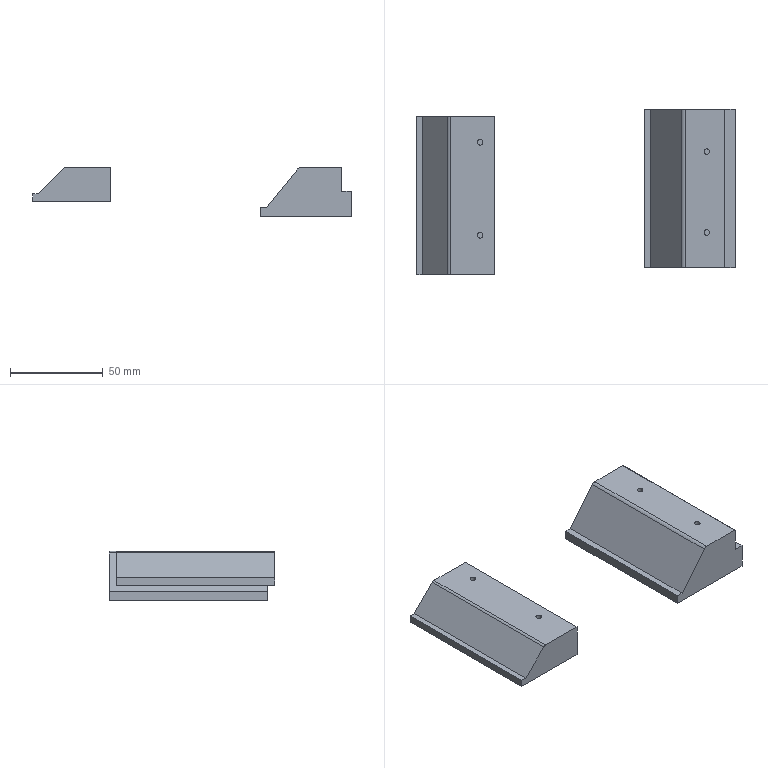NC program | NX | posted with a generic post | part box 171.319 x 88.841 x 26.598 mm
Lines 929 to 2519 of 2519:
(ZLEVEL_PROFILE , TOOL : D6R0.5)
N1838 T16 M6
N1840 G54
N1842 G17 G0 G90 X44.487 Y-6.407 S9500 M3
N1844 G43 Z30. H16
N1846 Z1.495
N1848 G94 G1 Z-0.005 F1000.
N1850 X44.029 Y-5.654
N1852 G3 X43.503 Y-5.365 R0.6
N1854 G1 X43.356 Y-5.369 F3000.
N1856 X42.665 Y-5.426
N1858 X42.5 Y-5.456
N1860 X-42.5
N1862 X-42.665 Y-5.426
N1864 X-43.356 Y-5.368
N1866 X-43.503 Y-5.365
N1868 X-43.504 Y-5.399 Z-0.01
N1870 X-42.5 Y-5.521
N1872 X42.5
N1874 X43.502 Y-5.404
N1876 X43.501 Y-5.445 Z-0.015
N1878 Y-5.478 Z-0.02
N1880 G2 X42.5 Y-5.61 R48.167
N1882 G1 X-42.5
N1884 G2 X-43.503 Y-5.463 R15.182
N1886 G1 X-43.502 Y-5.501 Z-0.025
N1888 X-43.5 Y-5.532 Z-0.03
N1890 X-42.5 Y-5.684
N1892 X42.5
N1894 X43.5 Y-5.547
N1896 Y-5.593 Z-0.037
N1898 Y-5.605 Z-0.043
N1900 G2 X42.5 Y-5.762 R67.588
N1902 G1 X-42.5
N1904 G2 X-43.5 Y-5.59 R13.651
N1906 G1 Y-5.641 Z-0.051
N1908 Y-5.658 Z-0.059
N1910 G3 X-42.5 Y-5.84 R11.561
N1912 G1 X42.5
N1914 X43.5 Y-5.675
N1916 Y-5.746 Z-0.069
N1918 Y-5.757 Z-0.078
N1920 X42.5 Y-5.92
N1922 X-42.5
N1924 X-42.665 Y-5.906
N1926 X-43.501 Y-5.74
N1928 Y-5.792 Z-0.089
N1930 Y-5.833 Z-0.1
N1932 X-42.5 Y-5.999
N1934 X42.5
N1936 X43.5 Y-5.852
N1938 Y-5.901 Z-0.113
N1940 Y-5.935 Z-0.125
N1942 X43.356 Y-5.938
N1944 X42.665 Y-6.054
N1946 X42.5 Y-6.08
N1948 X-42.5
N1950 X-43.501 Y-5.922
N1952 X-43.5 Y-5.96 Z-0.14
N1954 Y-6.013 Z-0.155
N1956 X-42.665 Y-6.145
N1958 X-42.5 Y-6.163
N1960 X42.5
N1962 X42.665 Y-6.145
N1964 X43.356 Y-6.025
N1966 X43.5 Y-6.022
N1968 Y-6.075 Z-0.171
N1970 Y-6.12 Z-0.187
N1972 X43.356 Y-6.123
N1974 X42.665 Y-6.241
N1976 X42.5 Y-6.248
N1978 X-42.5
N1980 X-42.665 Y-6.241
N1982 X-43.5 Y-6.115
N1984 Y-6.172 Z-0.206
N1986 Y-6.226 Z-0.224
N1988 X-43.356 Y-6.229
N1990 X-42.665 Y-6.323
N1992 X-42.5 Y-6.332
N1994 X42.5
N1996 X43.356 Y-6.229
N1998 X43.5 Y-6.226
N2000 Y-6.27 Z-0.244
N2002 Y-6.304 Z-0.264
N2004 X43.356 Y-6.306
N2006 X42.5 Y-6.416
N2008 X-42.5
N2010 X-43.356 Y-6.306
N2012 X-43.5 Y-6.304
N2014 Y-6.354 Z-0.286
N2016 Y-6.388 Z-0.308
N2018 X-43.356 Y-6.39
N2020 X-42.5 Y-6.5
N2022 X42.5
N2024 X43.356 Y-6.39
N2026 X43.5 Y-6.388
N2028 Y-6.435 Z-0.329
N2030 Y-6.469 Z-0.35
N2032 X43.356 Y-6.472
N2034 X42.5 Y-6.574
N2036 X-42.5
N2038 X-42.665 Y-6.569
N2040 X-43.356 Y-6.472
N2042 X-43.5 Y-6.469
N2044 Y-6.513 Z-0.371
N2046 Y-6.548 Z-0.391
N2048 G2 X-42.5 Y-6.641 R11.977
N2050 G1 X42.5
N2052 G2 X43.5 Y-6.548 R11.975
N2054 G1 Y-6.597 Z-0.416
N2056 Y-6.637 Z-0.44
N2058 X42.5 Y-6.714
N2060 X-42.5
N2062 X-43.5 Y-6.637
N2064 Y-6.677 Z-0.468
N2066 Y-6.714 Z-0.496
N2068 X-43.356 Y-6.717
N2070 X-42.665 Y-6.784
N2072 X-42.5 Y-6.792
N2074 X42.5
N2076 X42.665 Y-6.784
N2078 X43.356 Y-6.717
N2080 X43.5 Y-6.714
N2082 Y-6.755 Z-0.525
N2084 Y-6.788 Z-0.555
N2086 X43.356 Y-6.791
N2088 X42.5 Y-6.869
N2090 X-42.5
N2092 X-43.5 Y-6.79
N2094 Y-6.832 Z-0.587
N2096 Y-6.868 Z-0.618
N2098 X-42.5 Y-6.944
N2100 X42.5
N2102 X43.5 Y-6.865
N2104 Y-6.908 Z-0.651
N2106 Y-6.942 Z-0.684
N2108 X42.5 Y-7.016
N2110 X-42.5
N2112 X-43.356 Y-6.947
N2114 X-43.5 Y-6.945
N2116 Y-6.992 Z-0.717
N2118 Y-7.018 Z-0.751
N2120 X-43.356 Y-7.02
N2122 X-42.5 Y-7.084
N2124 X42.5
N2126 X43.5 Y-7.014
N2128 Y-7.062 Z-0.785
N2130 Y-7.088 Z-0.819
N2132 X43.356 Y-7.092
N2134 X42.5 Y-7.152
N2136 X-42.5
N2138 X-43.356 Y-7.094
N2140 X-43.5 Y-7.092
N2142 Y-7.139 Z-0.853
N2144 Y-7.167 Z-0.888
N2146 G2 X-42.5 Y-7.221 R12.469
N2148 G1 X42.5
N2150 X42.665 Y-7.217
N2152 X43.356 Y-7.167
N2154 X43.5 Y-7.163
N2156 Y-7.206 Z-0.923
N2158 Y-7.239 Z-0.958
N2160 X43.356 Y-7.244
N2162 X42.665 Y-7.289
N2164 X42.5 Y-7.291
N2166 X-42.5
N2168 G3 X-43.5 Y-7.243 R12.85
N2170 G1 Y-7.283 Z-0.993
N2172 Y-7.317 Z-1.028
N2174 G2 X-42.5 Y-7.362 R12.195
N2176 G1 X42.5
N2178 X42.665 Y-7.36
N2180 X43.356 Y-7.318
N2182 X43.5 Y-7.313
N2184 Y-7.351 Z-1.064
N2186 Y-7.386 Z-1.099
N2188 X43.356 Y-7.391
N2190 X42.665 Y-7.431
N2192 X42.5 Y-7.433
N2194 X-42.5
N2196 G3 X-43.5 Y-7.39 R11.828
N2198 G1 Y-7.43 Z-1.134
N2200 Y-7.463 Z-1.17
N2202 G2 X-42.5 Y-7.503 R11.483
N2204 G1 X42.5
N2206 X42.665 Y-7.502
N2208 X43.356 Y-7.464
N2210 X43.5 Y-7.46
N2212 Y-7.498 Z-1.205
N2214 Y-7.533 Z-1.241
N2216 X43.356 Y-7.537
N2218 X42.665 Y-7.572
N2220 X42.5 Y-7.574
N2222 X-42.5
N2224 G3 X-43.5 Y-7.536 R11.157
N2226 G1 Y-7.576 Z-1.276
N2228 Y-7.609 Z-1.311
N2230 G2 X-42.5 Y-7.645 R10.97
N2232 G1 X42.5
N2234 X42.665 Y-7.643
N2236 X43.356 Y-7.61
N2238 X43.5 Y-7.606
N2240 Y-7.644 Z-1.347
N2242 Y-7.679 Z-1.382
N2244 X43.356 Y-7.683
N2246 X42.665 Y-7.714
N2248 X42.5 Y-7.716
N2250 X-42.5
N2252 G3 X-43.5 Y-7.682 R11.802
N2254 G1 Y-7.722 Z-1.417
N2256 Y-7.755 Z-1.453
N2258 G2 X-42.5 Y-7.786 R12.772
N2260 G1 X42.5
N2262 X42.665 Y-7.785
N2264 X43.5 Y-7.752
N2266 Y-7.79 Z-1.488
N2268 Y-7.825 Z-1.523
N2270 X42.665 Y-7.855
N2272 X42.5 Y-7.857
N2274 X-42.5
N2276 G3 X-43.5 Y-7.828 R13.916
N2278 G1 Y-7.868 Z-1.559
N2280 Y-7.902 Z-1.594
N2282 X-43.356 Y-7.904
N2284 X-42.5 Y-7.928
N2286 X42.5
N2288 X43.5 Y-7.898
N2290 Y-7.936 Z-1.629
N2292 Y-7.971 Z-1.665
N2294 X43.356 Y-7.975
N2296 X42.5 Y-7.998
N2298 X-42.5
N2300 X-43.5 Y-7.975
N2302 Y-8.014 Z-1.7
N2304 Y-8.048 Z-1.736
N2306 X-42.5 Y-8.069
N2308 X42.5
N2310 X43.5 Y-8.044
N2312 Y-8.082 Z-1.771
N2314 Y-8.117 Z-1.806
N2316 X42.5 Y-8.14
N2318 X-42.5
N2320 X-43.5 Y-8.121
N2322 Y-8.161 Z-1.842
N2324 Y-8.194 Z-1.877
N2326 X-42.5 Y-8.211
N2328 X42.5
N2330 X43.5 Y-8.19
N2332 Y-8.228 Z-1.912
N2334 Y-8.263 Z-1.948
N2336 X42.5 Y-8.281
N2338 X-42.5
N2340 X-42.665 Y-8.276
N2342 X-43.5 Y-8.267
N2344 Y-8.307 Z-1.983
N2346 Y-8.339 Z-2.018
N2348 X-42.5 Y-8.352
N2350 X42.5
N2352 X43.356 Y-8.339
N2354 X43.5 Y-8.335
N2356 Y-8.374 Z-2.054
N2358 Y-8.407 Z-2.089
N2360 X43.356 Y-8.411
N2362 X42.5 Y-8.423
N2364 X-42.5
N2366 X-43.5 Y-8.411
N2368 Y-8.452 Z-2.124
N2370 Y-8.483 Z-2.16
N2372 X-42.5 Y-8.493
N2374 X42.5
N2376 X42.665 Y-8.492
N2378 X43.356 Y-8.483
N2380 X43.5 Y-8.479
N2382 Y-8.518 Z-2.195
N2384 Y-8.551 Z-2.23
N2386 X43.356 Y-8.555
N2388 X42.5 Y-8.564
N2390 X-42.5
N2392 X-43.5 Y-8.555
N2394 Y-8.594 Z-2.266
N2396 Y-8.627 Z-2.301
N2398 X-42.5 Y-8.635
N2400 X42.5
N2402 X43.356 Y-8.627
N2404 X43.5 Y-8.623
N2406 Y-8.66 Z-2.337
N2408 Y-8.694 Z-2.372
N2410 X43.356 Y-8.698
N2412 X42.5 Y-8.706
N2414 X-42.5
N2416 X-43.5 Y-8.698
N2418 Y-8.736 Z-2.407
N2420 Y-8.769 Z-2.443
N2422 X-42.665 Y-8.774
N2424 X-42.5 Y-8.776
N2426 X42.5
N2428 X43.356 Y-8.769
N2430 X43.5 Y-8.765
N2432 Y-8.803 Z-2.478
N2434 Y-8.837 Z-2.513
N2436 X43.356 Y-8.84
N2438 X42.5 Y-8.847
N2440 X-42.5
N2442 X-42.665 Y-8.845
N2444 X-43.5 Y-8.84
N2446 Y-8.878 Z-2.549
N2448 Y-8.911 Z-2.584
N2450 X-42.5 Y-8.918
N2452 X42.5
N2454 X43.356 Y-8.912
N2456 X43.5 Y-8.908
N2458 Y-8.945 Z-2.619
N2460 Y-8.979 Z-2.655
N2462 X43.356 Y-8.983
N2464 X42.5 Y-8.988
N2466 X-42.5
N2468 X-43.5 Y-8.983
N2470 Y-9.02 Z-2.69
N2472 Y-9.053 Z-2.725
N2474 X-42.5 Y-9.059
N2476 X42.5
N2478 X43.356 Y-9.054
N2480 X43.5 Y-9.05
N2482 Y-9.088 Z-2.761
N2484 Y-9.122 Z-2.796
N2486 X43.356 Y-9.125
N2488 X42.5 Y-9.13
N2490 X-42.5
N2492 X-42.665 Y-9.128
N2494 X-43.356 Y-9.127
N2496 X-43.5 Y-9.124
N2498 Y-9.162 Z-2.832
N2500 Y-9.195 Z-2.867
N2502 X-43.356 Y-9.198
N2504 X-42.665
N2506 X-42.5 Y-9.2
N2508 X42.5
N2510 X43.356 Y-9.197
N2512 X43.5 Y-9.193
N2514 Y-9.231 Z-2.902
N2516 Y-9.264 Z-2.938
N2518 X43.356 Y-9.268
N2520 X42.5 Y-9.271
N2522 X-42.5
N2524 X-42.665 Y-9.269
N2526 X-43.356
N2528 X-43.5 Y-9.266
N2530 Y-9.304 Z-2.973
N2532 Y-9.337 Z-3.008
N2534 X-43.356 Y-9.34
N2536 X-42.665
N2538 X-42.5 Y-9.342
N2540 X42.5
N2542 X43.356 Y-9.339
N2544 X43.5 Y-9.335
N2546 Y-9.373 Z-3.044
N2548 Y-9.406 Z-3.079
N2550 X43.356 Y-9.41
N2552 X42.5 Y-9.413
N2554 X-42.5
N2556 X-42.665 Y-9.411
N2558 X-43.356
N2560 X-43.5 Y-9.408
N2562 Y-9.446 Z-3.114
N2564 Y-9.479 Z-3.15
N2566 X-43.356 Y-9.482
N2568 X-42.5 Y-9.483
N2570 X42.5
N2572 X43.356 Y-9.481
N2574 X43.5 Y-9.478
N2576 Y-9.516 Z-3.185
N2578 Y-9.549 Z-3.22
N2580 X43.356 Y-9.552
N2582 X42.5 Y-9.554
N2584 X-42.5
N2586 X-43.356 Y-9.553
N2588 X-43.5 Y-9.55
N2590 Y-9.588 Z-3.256
N2592 Y-9.621 Z-3.291
N2594 X-43.356 Y-9.624
N2596 X-42.5 Y-9.625
N2598 X42.5
N2600 X43.356 Y-9.623
N2602 X43.5 Y-9.62
N2604 Y-9.658 Z-3.326
N2606 Y-9.691 Z-3.362
N2608 X43.356 Y-9.694
N2610 X42.5 Y-9.695
N2612 X-42.5
N2614 X-43.356 Y-9.694
N2616 X-43.5 Y-9.692
N2618 Y-9.73 Z-3.397
N2620 Y-9.762 Z-3.433
N2622 X-43.356 Y-9.765
N2624 X-42.5 Y-9.766
N2626 X42.5
N2628 X43.356 Y-9.765
N2630 X43.5 Y-9.762
N2632 Y-9.8 Z-3.468
N2634 Y-9.833 Z-3.503
N2636 X43.356 Y-9.836
N2638 X42.5 Y-9.837
N2640 X-42.5
N2642 X-43.356 Y-9.836
N2644 X-43.5 Y-9.833
N2646 Y-9.872 Z-3.539
N2648 Y-9.904 Z-3.574
N2650 X-43.356 Y-9.907
N2652 X-42.5 Y-9.908
N2654 X42.5
N2656 X43.356 Y-9.907
N2658 X43.5 Y-9.903
N2660 Y-9.942 Z-3.609
N2662 Y-9.974 Z-3.645
N2664 X43.356 Y-9.977
N2666 X42.5 Y-9.978
N2668 X-42.5
N2670 X-43.356
N2672 X-43.5 Y-9.975
N2674 Y-10.013 Z-3.68
N2676 Y-10.046 Z-3.715
N2678 X-43.356 Y-10.049
N2680 X-42.5
N2682 X42.5
N2684 X43.356 Y-10.048
N2686 X43.5 Y-10.045
N2688 Y-10.083 Z-3.751
N2690 Y-10.116 Z-3.786
N2692 X43.356 Y-10.119
N2694 X42.5 Y-10.12
N2696 X-42.5
N2698 X-43.356 Y-10.119
N2700 X-43.5 Y-10.116
N2702 Y-10.155 Z-3.821
N2704 Y-10.187 Z-3.857
N2706 X-43.356 Y-10.19
N2708 X-42.5
N2710 X42.5
N2712 X43.356
N2714 X43.5 Y-10.187
N2716 Y-10.225 Z-3.892
N2718 Y-10.258 Z-3.928
N2720 X43.356 Y-10.261
N2722 X42.5
N2724 X-42.5
N2726 X-43.356
N2728 X-43.5 Y-10.258
N2730 Y-10.296 Z-3.963
N2732 Y-10.329 Z-3.998
N2734 X-43.356 Y-10.332
N2736 X-42.5
N2738 X42.5
N2740 X43.356 Y-10.331
N2742 X43.5 Y-10.328
N2744 Y-10.367 Z-4.034
N2746 Y-10.399 Z-4.069
N2748 X43.356 Y-10.402
N2750 X42.5 Y-10.403
N2752 X-42.5
N2754 X-43.356 Y-10.402
N2756 X-43.5 Y-10.399
N2758 Y-10.438 Z-4.104
N2760 Y-10.47 Z-4.14
N2762 X-43.356 Y-10.473
N2764 X-42.5
N2766 X42.5
N2768 X43.356
N2770 X43.5 Y-10.47
N2772 Y-10.508 Z-4.175
N2774 Y-10.541 Z-4.21
N2776 X43.356 Y-10.544
N2778 X42.5
N2780 X-42.5
N2782 X-43.356
N2784 X-43.5 Y-10.541
N2786 Y-10.579 Z-4.246
N2788 Y-10.612 Z-4.281
N2790 X-43.356 Y-10.615
N2792 X-42.5
N2794 X42.5
N2796 X43.356 Y-10.614
N2798 X43.5 Y-10.611
N2800 Y-10.65 Z-4.316
N2802 Y-10.682 Z-4.352
N2804 X43.356 Y-10.685
N2806 X42.5
N2808 X-42.5
N2810 X-43.356
N2812 X-43.5 Y-10.682
N2814 Y-10.721 Z-4.387
N2816 Y-10.753 Z-4.422
N2818 X-43.356 Y-10.756
N2820 X-42.5
N2822 X42.5
N2824 X43.356
N2826 X43.5 Y-10.753
N2828 Y-10.791 Z-4.458
N2830 Y-10.824 Z-4.493
N2832 X43.356 Y-10.827
N2834 X42.5
N2836 X-42.5
N2838 X-43.356
N2840 X-43.5 Y-10.824
N2842 Y-10.862 Z-4.529
N2844 Y-10.894 Z-4.564
N2846 X-43.356 Y-10.897
N2848 X-42.5 Y-10.898
N2850 X42.5
N2852 X43.356 Y-10.897
N2854 X43.5 Y-10.894
N2856 Y-10.933 Z-4.599
N2858 Y-10.965 Z-4.635
N2860 X43.356 Y-10.968
N2862 X42.5
N2864 X-42.5
N2866 X-43.356
N2868 X-43.5 Y-10.965
N2870 Y-11.004 Z-4.67
N2872 Y-11.036 Z-4.705
N2874 X-43.356 Y-11.039
N2876 X-42.5
N2878 X42.5
N2880 X43.356
N2882 X43.5 Y-11.036
N2884 Y-11.074 Z-4.741
N2886 Y-11.107 Z-4.776
N2888 X43.356 Y-11.11
N2890 X42.5
N2892 X-42.5
N2894 X-43.356
N2896 X-43.5 Y-11.107
N2898 Y-11.145 Z-4.811
N2900 Y-11.177 Z-4.847
N2902 X-43.356 Y-11.18
N2904 X-42.5
N2906 X42.5
N2908 X43.356
N2910 X43.5 Y-11.177
N2912 Y-11.216 Z-4.882
N2914 Y-11.248 Z-4.917
N2916 X43.356 Y-11.251
N2918 X42.5
N2920 X-42.5
N2922 X-43.356
N2924 X-43.5 Y-11.248
N2926 Y-11.286 Z-4.953
N2928 Y-11.319 Z-4.988
N2930 X-43.356 Y-11.322
N2932 X-42.5
N2934 X42.5
N2936 X43.356
N2938 X43.5 Y-11.319
N2940 Y-11.357 Z-5.024
N2942 Y-11.39 Z-5.059
N2944 X43.356 Y-11.392
N2946 X42.5 Y-11.393
N2948 X-42.5
N2950 X-43.356
N2952 X-43.5 Y-11.39
N2954 Y-11.428 Z-5.094
N2956 Y-11.46 Z-5.13
N2958 X-43.356 Y-11.463
N2960 X-42.5
N2962 X42.5
N2964 X43.356
N2966 X43.5 Y-11.46
N2968 Y-11.499 Z-5.165
N2970 Y-11.531 Z-5.2
N2972 X43.356 Y-11.534
N2974 X42.5
N2976 X-42.5
N2978 X-43.356
N2980 X-43.5 Y-11.531
N2982 Y-11.569 Z-5.236
N2984 Y-11.602 Z-5.271
N2986 X-43.356 Y-11.605
N2988 X-42.5
N2990 X42.5
N2992 X43.356
N2994 X43.5 Y-11.602
N2996 Y-11.64 Z-5.306
N2998 Y-11.672 Z-5.342
N3000 X43.356 Y-11.675
N3002 X42.5
N3004 X-42.5
N3006 X-43.356
N3008 X-43.5 Y-11.672
N3010 Y-11.711 Z-5.377
N3012 Y-11.744 Z-5.412
N3014 X-43.356 Y-11.746
N3016 X-42.5
N3018 X42.5
N3020 X43.356
N3022 X43.5 Y-11.744
N3024 Y-11.781 Z-5.448
N3026 Y-11.814 Z-5.483
N3028 X43.356 Y-11.817
N3030 X42.5
N3032 X-42.5
N3034 X-43.356
N3036 X-43.5 Y-11.814
N3038 Y-11.852 Z-5.518
N3040 Y-11.885 Z-5.554
N3042 X-43.356 Y-11.888
N3044 X-42.5
N3046 X42.5
N3048 X43.356
N3050 X43.5 Y-11.885
N3052 Y-11.923 Z-5.589
N3054 Y-11.955 Z-5.625
N3056 X43.356 Y-11.958
N3058 X42.5
N3060 X-42.5
N3062 X-43.356
N3064 X-43.5 Y-11.955
N3066 Y-11.994 Z-5.66
N3068 Y-12.026 Z-5.695
N3070 X-43.356 Y-12.029
N3072 X-42.5
N3074 X42.5
N3076 X43.356
N3078 X43.5 Y-12.026
N3080 Y-12.064 Z-5.731
N3082 Y-12.097 Z-5.766
N3084 X43.356 Y-12.1
N3086 X42.5
N3088 X-42.5
N3090 X-43.356
N3092 X-43.5 Y-12.097
N3094 Y-12.135 Z-5.801
N3096 Y-12.167 Z-5.837
N3098 X-43.356 Y-12.17
N3100 X-42.5
N3102 X42.5
N3104 X43.356
N3106 X43.5 Y-12.167
N3108 Y-12.206 Z-5.872
N3110 Y-12.238 Z-5.907
N3112 X43.356 Y-12.241
N3114 X42.5
N3116 X-42.5
N3118 X-43.356
N3120 X-43.5 Y-12.238
N3122 Y-12.276 Z-5.943
N3124 Y-12.309 Z-5.978
N3126 X-43.356 Y-12.312
N3128 X-42.5
N3130 X42.5
N3132 X43.356
N3134 X43.5 Y-12.309
N3136 Y-12.347 Z-6.013
N3138 Y-12.38 Z-6.049
N3140 X43.356 Y-12.383
N3142 X42.5
N3144 X-42.5
N3146 X-43.356
N3148 X-43.5 Y-12.38
N3150 Y-12.418 Z-6.084
N3152 Y-12.45 Z-6.12
N3154 X-43.356 Y-12.453
N3156 X-42.5
N3158 X42.5
N3160 X43.356
N3162 X43.5 Y-12.45
N3164 Y-12.489 Z-6.155
N3166 Y-12.521 Z-6.19
N3168 X43.356 Y-12.524
N3170 X42.5
N3172 X-42.5
N3174 X-43.356
N3176 X-43.5 Y-12.521
N3178 Y-12.559 Z-6.226
N3180 Y-12.592 Z-6.261
N3182 X-43.356 Y-12.595
N3184 X-42.5
N3186 X42.5
N3188 X43.356
N3190 X43.5 Y-12.592
N3192 Y-12.63 Z-6.296
N3194 Y-12.662 Z-6.332
N3196 X43.356 Y-12.665
N3198 X42.5
N3200 X-42.5
N3202 X-43.356
N3204 X-43.5 Y-12.662
N3206 Y-12.701 Z-6.367
N3208 Y-12.733 Z-6.402
N3210 X-43.356 Y-12.736
N3212 X-42.5
N3214 X42.5
N3216 X43.356
N3218 X43.5 Y-12.733
N3220 Y-12.771 Z-6.438
N3222 Y-12.804 Z-6.473
N3224 X43.356 Y-12.807
N3226 X42.5
N3228 X-42.5
N3230 X-43.356
N3232 X-43.5 Y-12.804
N3234 Y-12.842 Z-6.508
N3236 Y-12.875 Z-6.544
N3238 X-43.356 Y-12.877
N3240 X-42.5
N3242 X42.5
N3244 X43.356
N3246 X43.5 Y-12.875
N3248 Y-12.913 Z-6.579
N3250 Y-12.945 Z-6.614
N3252 X43.356 Y-12.948
N3254 X42.5
N3256 X-42.5
N3258 X-43.356
N3260 X-43.5 Y-12.945
N3262 Y-12.984 Z-6.65
N3264 Y-13.016 Z-6.685
N3266 X-43.356 Y-13.019
N3268 X-42.5
N3270 X42.5
N3272 X43.356
N3274 X43.5 Y-13.016
N3276 Y-13.054 Z-6.721
N3278 Y-13.087 Z-6.756
N3280 X43.356 Y-13.09
N3282 X42.5
N3284 X-42.5
N3286 X-43.356
N3288 X-43.5 Y-13.087
N3290 Y-13.125 Z-6.791
N3292 Y-13.157 Z-6.827
N3294 X-43.356 Y-13.16
N3296 X-42.5
N3298 X42.5
N3300 X43.356
N3302 X43.5 Y-13.157
N3304 Y-13.196 Z-6.862
N3306 Y-13.228 Z-6.897
N3308 X43.356 Y-13.231
N3310 X42.5
N3312 X-42.5
N3314 X-43.356
N3316 X-43.5 Y-13.228
N3318 Y-13.266 Z-6.933
N3320 Y-13.299 Z-6.968
N3322 X-43.356 Y-13.302
N3324 X-42.5
N3326 X42.5
N3328 X43.356
N3330 X43.5 Y-13.299
N3332 Y-13.337 Z-7.003
N3334 Y-13.37 Z-7.039
N3336 X43.356 Y-13.372
N3338 X42.5
N3340 X-42.5
N3342 X-43.356
N3344 X-43.5 Y-13.37
N3346 Y-13.408 Z-7.074
N3348 Y-13.44 Z-7.109
N3350 X-43.356 Y-13.443
N3352 X-42.5
N3354 X42.5
N3356 X43.356
N3358 X43.5 Y-13.44
N3360 Y-13.479 Z-7.145
N3362 Y-13.511 Z-7.18
N3364 X43.356 Y-13.514
N3366 X42.5
N3368 X-42.5
N3370 X-43.356
N3372 X-43.5 Y-13.511
N3374 Y-13.549 Z-7.216
N3376 Y-13.582 Z-7.251
N3378 X-43.356 Y-13.585
N3380 X-42.5
N3382 X42.5
N3384 X43.356
N3386 X43.5 Y-13.582
N3388 Y-13.62 Z-7.286
N3390 Y-13.652 Z-7.322
N3392 X43.356 Y-13.655
N3394 X42.5
N3396 X-42.5
N3398 X-43.356
N3400 X-43.5 Y-13.652
N3402 Y-13.691 Z-7.357
N3404 Y-13.723 Z-7.392
N3406 X-43.356 Y-13.726
N3408 X-42.5
N3410 X42.5
N3412 X43.356
N3414 X43.5 Y-13.723
N3416 Y-13.761 Z-7.428
N3418 Y-13.794 Z-7.463
N3420 X43.356 Y-13.797
N3422 X42.5
N3424 X-42.5
N3426 X-43.356
N3428 X-43.5 Y-13.794
N3430 Y-13.832 Z-7.498
N3432 Y-13.864 Z-7.534
N3434 X-43.356 Y-13.867
N3436 X-42.5
N3438 X42.5
N3440 X43.356
N3442 X43.5 Y-13.864
N3444 Y-13.903 Z-7.569
N3446 Y-13.935 Z-7.604
N3448 X43.356 Y-13.938
N3450 X42.5
N3452 X-42.5
N3454 X-43.356
N3456 X-43.5 Y-13.935
N3458 Y-13.974 Z-7.64
N3460 Y-14.006 Z-7.675
N3462 X-43.356 Y-14.009
N3464 X-42.5
N3466 X42.5
N3468 X43.356
N3470 X43.5 Y-14.006
N3472 Y-14.044 Z-7.711
N3474 Y-14.077 Z-7.746
N3476 X43.356 Y-14.08
N3478 X42.5
N3480 X-42.5
N3482 X-43.356
N3484 X-43.5 Y-14.077
N3486 Y-14.115 Z-7.781
N3488 X-43.499 Y-14.147 Z-7.817
N3490 X-43.356 Y-14.15
N3492 X-42.5
N3494 X42.5
N3496 X43.356
N3498 X43.5 Y-14.147
N3500 Y-14.186 Z-7.852
N3502 Y-14.218 Z-7.887
N3504 X43.356 Y-14.221
N3506 X42.5
N3508 X-42.5
N3510 X-43.356
N3512 X-43.499 Y-14.218
N3514 Y-14.256 Z-7.923
N3516 Y-14.289 Z-7.958
N3518 X-43.356 Y-14.292
N3520 X-42.5
N3522 X42.5
N3524 X43.356
N3526 X43.5 Y-14.289
N3528 Y-14.327 Z-7.993
N3530 Y-14.359 Z-8.029
N3532 X43.356 Y-14.362
N3534 X42.5
N3536 X-42.5
N3538 X-43.356
N3540 X-43.499 Y-14.359
N3542 Y-14.398 Z-8.064
N3544 Y-14.43 Z-8.099
N3546 X-43.356 Y-14.433
N3548 X-42.5
N3550 X42.5
N3552 X43.356
N3554 X43.5 Y-14.43
N3556 Y-14.468 Z-8.135
N3558 X43.499 Y-14.501 Z-8.17
N3560 X43.356 Y-14.504
N3562 X42.5
N3564 X-42.5
N3566 X-43.356
N3568 X-43.499 Y-14.501
N3570 Y-14.539 Z-8.205
N3572 Y-14.572 Z-8.241
N3574 X-43.356 Y-14.575
N3576 X-42.5
N3578 X42.5
N3580 X43.356
N3582 X43.499 Y-14.572
N3584 Y-14.61 Z-8.276
N3586 Y-14.642 Z-8.312
N3588 X43.356 Y-14.645
N3590 X42.5
N3592 X-42.5
N3594 X-43.356
N3596 X-43.499 Y-14.642
N3598 Y-14.681 Z-8.347
N3600 Y-14.713 Z-8.382
N3602 X-43.356 Y-14.716
N3604 X-42.5
N3606 X42.5
N3608 X43.356
N3610 X43.499 Y-14.713
N3612 Y-14.751 Z-8.418
N3614 Y-14.784 Z-8.453
N3616 X43.356 Y-14.787
N3618 X-43.356
N3620 X-43.499 Y-14.784
N3622 Y-14.822 Z-8.488
N3624 Y-14.854 Z-8.524
N3626 X-43.356 Y-14.857
N3628 X43.356
N3630 X43.499 Y-14.854
N3632 Y-14.893 Z-8.559
N3634 Y-14.925 Z-8.594
N3636 X43.356 Y-14.928
N3638 X-43.356
N3640 X-43.499 Y-14.925
N3642 Y-14.963 Z-8.63
N3644 Y-14.996 Z-8.665
N3646 X-43.356 Y-14.999
N3648 X43.356
N3650 X43.499 Y-14.996
N3652 Y-15.034 Z-8.7
N3654 Y-15.067 Z-8.736
N3656 X43.356 Y-15.07
N3658 X-43.356
N3660 X-43.499 Y-15.067
N3662 Y-15.105 Z-8.771
N3664 Y-15.137 Z-8.807
N3666 X-43.356 Y-15.14
N3668 X43.356
N3670 X43.499 Y-15.137
N3672 Y-15.176 Z-8.842
N3674 Y-15.208 Z-8.877
N3676 X43.356 Y-15.211
N3678 X-43.356
N3680 X-43.499 Y-15.208
N3682 Y-15.246 Z-8.913
N3684 Y-15.279 Z-8.948
N3686 X-43.356 Y-15.282
N3688 X42.5
N3690 X43.356
N3692 X43.499 Y-15.279
N3694 Y-15.317 Z-8.983
N3696 Y-15.349 Z-9.019
N3698 X43.356 Y-15.352
N3700 X42.5
N3702 X-43.356
N3704 X-43.499 Y-15.349
N3706 Y-15.388 Z-9.054
N3708 Y-15.42 Z-9.089
N3710 X-43.356 Y-15.423
N3712 X42.5
N3714 X43.356
N3716 X43.499 Y-15.42
N3718 Y-15.458 Z-9.125
N3720 Y-15.491 Z-9.16
N3722 X43.356 Y-15.494
N3724 X42.5
N3726 X-43.356
N3728 X-43.499 Y-15.491
N3730 Y-15.529 Z-9.195
N3732 Y-15.562 Z-9.231
N3734 X-43.356 Y-15.565
N3736 X42.5
N3738 X43.356
N3740 X43.499 Y-15.562
N3742 Y-15.6 Z-9.266
N3744 Y-15.632 Z-9.301
N3746 X43.356 Y-15.635
N3748 X42.5
N3750 X-43.356
N3752 X-43.499 Y-15.632
N3754 Y-15.671 Z-9.337
N3756 Y-15.703 Z-9.372
N3758 X-43.356 Y-15.706
N3760 X42.5
N3762 X43.356
N3764 X43.499 Y-15.703
N3766 Y-15.741 Z-9.408
N3768 Y-15.774 Z-9.443
N3770 X43.356 Y-15.777
N3772 X42.5
N3774 X-43.356
N3776 X-43.499 Y-15.774
N3778 Y-15.812 Z-9.478
N3780 Y-15.844 Z-9.514
N3782 X-43.356 Y-15.847
N3784 X42.5
N3786 X43.356
N3788 X43.499 Y-15.844
N3790 X43.498 Y-15.883 Z-9.549
N3792 Y-15.915 Z-9.584
N3794 X43.356 Y-15.918
N3796 X42.5
N3798 X-43.356
N3800 X-43.498 Y-15.915
N3802 Y-15.953 Z-9.62
N3804 Y-15.986 Z-9.655
N3806 X-43.356 Y-15.989
N3808 X42.5
N3810 X43.356
N3812 X43.498 Y-15.986
N3814 Y-16.024 Z-9.69
N3816 Y-16.057 Z-9.726
N3818 X43.356 Y-16.06
N3820 X42.5
N3822 X-43.356
N3824 X-43.498 Y-16.057
N3826 Y-16.095 Z-9.761
N3828 Y-16.127 Z-9.796
N3830 X-43.356 Y-16.13
N3832 X42.5
N3834 X43.356
N3836 X43.498 Y-16.127
N3838 Y-16.166 Z-9.832
N3840 Y-16.198 Z-9.867
N3842 X43.356 Y-16.201
N3844 X42.5
N3846 X-43.356
N3848 X-43.498 Y-16.198
N3850 Y-16.236 Z-9.903
N3852 Y-16.269 Z-9.938
N3854 X-43.356 Y-16.272
N3856 X42.5
N3858 X43.356
N3860 X43.498 Y-16.269
N3862 Y-16.307 Z-9.973
N3864 Y-16.339 Z-10.009
N3866 X43.356 Y-16.342
N3868 X42.5
N3870 X-43.356
N3872 X-43.498 Y-16.339
N3874 Y-16.378 Z-10.044
N3876 Y-16.41 Z-10.079
N3878 X-43.356 Y-16.413
N3880 X42.5
N3882 X43.356
N3884 X43.498 Y-16.41
N3886 Y-16.448 Z-10.115
N3888 Y-16.481 Z-10.15
N3890 X43.356 Y-16.484
N3892 X42.5
N3894 X-43.356
N3896 X-43.498 Y-16.481
N3898 Y-16.519 Z-10.185
N3900 Y-16.552 Z-10.221
N3902 X-43.356 Y-16.554
N3904 X42.5
N3906 X43.356
N3908 X43.498 Y-16.552
N3910 Y-16.59 Z-10.256
N3912 X43.497 Y-16.622 Z-10.291
N3914 X43.356 Y-16.625
N3916 X42.5
N3918 X-43.356
N3920 X-43.498 Y-16.622
N3922 X-43.497 Y-16.661 Z-10.327
N3924 Y-16.693 Z-10.362
N3926 X-43.356 Y-16.696
N3928 X42.5
N3930 X43.356
N3932 X43.497 Y-16.693
N3934 Y-16.731 Z-10.397
N3936 Y-16.764 Z-10.433
N3938 X43.356 Y-16.767
N3940 X42.5
N3942 X-43.356
N3944 X-43.497 Y-16.764
N3946 Y-16.802 Z-10.468
N3948 Y-16.834 Z-10.504
N3950 X-43.356 Y-16.837
N3952 X42.5
N3954 X43.356
N3956 X43.497 Y-16.834
N3958 Y-16.873 Z-10.539
N3960 Y-16.905 Z-10.574
N3962 X43.356 Y-16.908
N3964 X42.5
N3966 X-43.356
N3968 X-43.497 Y-16.905
N3970 Y-16.943 Z-10.61
N3972 Y-16.976 Z-10.645
N3974 X-43.356 Y-16.979
N3976 X42.5
N3978 X43.356
N3980 X43.497 Y-16.976
N3982 Y-17.014 Z-10.68
N3984 X43.496 Y-17.046 Z-10.716
N3986 X43.356 Y-17.049
N3988 X42.5
N3990 X-43.356
N3992 X-43.496 Y-17.046
N3994 Y-17.085 Z-10.751
N3996 Y-17.117 Z-10.786
N3998 X-43.356 Y-17.12
N4000 X42.5
N4002 X43.356
N4004 X43.496 Y-17.117
N4006 Y-17.156 Z-10.822
N4008 Y-17.188 Z-10.857
N4010 X43.356 Y-17.191
N4012 X42.5
N4014 X-43.356
N4016 X-43.496 Y-17.188
N4018 Y-17.226 Z-10.892
N4020 Y-17.259 Z-10.928
N4022 X-43.356 Y-17.262
N4024 X42.5
N4026 X43.356
N4028 X43.496 Y-17.259
N4030 Y-17.297 Z-10.963
N4032 Y-17.329 Z-10.999
N4034 X43.356 Y-17.332
N4036 X42.5
N4038 X-43.356
N4040 X-43.496 Y-17.329
N4042 X-43.495 Y-17.368 Z-11.034
N4044 Y-17.4 Z-11.069
N4046 X-43.356 Y-17.403
N4048 X42.5
N4050 X43.356
N4052 X43.495 Y-17.4
N4054 Y-17.438 Z-11.105
N4056 Y-17.471 Z-11.14
N4058 X43.356 Y-17.474
N4060 X42.5
N4062 X-43.356
N4064 X-43.495 Y-17.471
N4066 Y-17.509 Z-11.175
N4068 Y-17.541 Z-11.211
N4070 X-43.356 Y-17.544
N4072 X42.5
N4074 X43.356
N4076 X43.495 Y-17.541
N4078 Y-17.58 Z-11.246
N4080 Y-17.613 Z-11.281
N4082 X43.356 Y-17.615
N4084 X42.5
N4086 X-43.356
N4088 X-43.495 Y-17.613
N4090 Y-17.651 Z-11.317
N4092 Y-17.683 Z-11.352
N4094 X-43.356 Y-17.686
N4096 X42.5
N4098 X43.356
N4100 X43.495 Y-17.683
N4102 Y-17.721 Z-11.387
N4104 X43.494 Y-17.754 Z-11.423
N4106 X43.356 Y-17.757
N4108 X42.5
N4110 X-43.356
N4112 X-43.494 Y-17.754
N4114 Y-17.792 Z-11.458
N4116 Y-17.824 Z-11.493
N4118 X-43.356 Y-17.827
N4120 X42.5
N4122 X43.356
N4124 X43.494 Y-17.824
N4126 Y-17.863 Z-11.529
N4128 Y-17.895 Z-11.564
N4130 X43.356 Y-17.898
N4132 X42.5
N4134 X-43.356
N4136 X-43.494 Y-17.895
N4138 Y-17.933 Z-11.6
N4140 Y-17.966 Z-11.635
N4142 X-43.356 Y-17.969
N4144 X42.5
N4146 X43.356
N4148 X43.494 Y-17.966
N4150 Y-18.004 Z-11.67
N4152 X43.493 Y-18.036 Z-11.706
N4154 X43.356 Y-18.039
N4156 X42.5
N4158 X-43.356
N4160 X-43.493 Y-18.036
N4162 Y-18.075 Z-11.741
N4164 Y-18.107 Z-11.776
N4166 X-43.356 Y-18.11
N4168 X42.5
N4170 X43.356
N4172 X43.493 Y-18.107
N4174 Y-18.145 Z-11.812
N4176 Y-18.178 Z-11.847
N4178 X43.356 Y-18.181
N4180 X42.5
N4182 X-43.356
N4184 X-43.493 Y-18.178
N4186 X-43.492 Y-18.216 Z-11.882
N4188 Y-18.249 Z-11.918
N4190 X-43.356 Y-18.252
N4192 X42.5
N4194 X43.356
N4196 X43.492 Y-18.249
N4198 Y-18.287 Z-11.953
N4200 Y-18.319 Z-11.988
N4202 X43.356 Y-18.322
N4204 X42.5
N4206 X-43.356
N4208 X-43.492 Y-18.319
N4210 Y-18.358 Z-12.024
N4212 Y-18.39 Z-12.059
N4214 X-43.356 Y-18.393
N4216 X42.5
N4218 X43.356
N4220 X43.492 Y-18.39
N4222 X43.491 Y-18.428 Z-12.095
N4224 Y-18.461 Z-12.13
N4226 X43.356 Y-18.464
N4228 X42.5
N4230 X-43.356
N4232 X-43.491 Y-18.461
N4234 Y-18.499 Z-12.165
N4236 Y-18.531 Z-12.201
N4238 X-43.356 Y-18.534
N4240 X42.5
N4242 X43.356
N4244 X43.491 Y-18.531
N4246 Y-18.57 Z-12.236
N4248 X43.49 Y-18.602 Z-12.271
N4250 X43.356 Y-18.605
N4252 X42.5
N4254 X-43.356
N4256 X-43.49 Y-18.602
N4258 Y-18.64 Z-12.307
N4260 Y-18.673 Z-12.342
N4262 X-43.356 Y-18.676
N4264 X42.5
N4266 X43.356
N4268 X43.49 Y-18.673
N4270 Y-18.711 Z-12.377
N4272 Y-18.743 Z-12.413
N4274 X43.356 Y-18.747
N4276 X42.5
N4278 X-43.356
N4280 X-43.489 Y-18.744
N4282 Y-18.782 Z-12.448
N4284 Y-18.814 Z-12.483
N4286 X-43.356 Y-18.817
N4288 X42.5
N4290 X43.356
N4292 X43.489 Y-18.814
N4294 Y-18.853 Z-12.519
N4296 Y-18.885 Z-12.554
N4298 X43.356 Y-18.888
N4300 X42.5
N4302 X-43.356
N4304 X-43.489 Y-18.885
N4306 X-43.488 Y-18.923 Z-12.589
N4308 Y-18.956 Z-12.625
N4310 X-43.356 Y-18.959
N4312 X42.5
N4314 X43.356
N4316 X43.488 Y-18.956
N4318 Y-18.994 Z-12.66
N4320 Y-19.026 Z-12.696
N4322 X43.356 Y-19.029
N4324 X42.5
N4326 X-43.356
N4328 X-43.488 Y-19.026
N4330 Y-19.065 Z-12.731
N4332 X-43.487 Y-19.097 Z-12.766
N4334 X-43.356 Y-19.1
N4336 X42.5
N4338 X43.356
N4340 X43.487 Y-19.097
N4342 Y-19.135 Z-12.802
N4344 Y-19.168 Z-12.837
N4346 X43.356 Y-19.171
N4348 X42.5
N4350 X-43.356
N4352 X-43.487 Y-19.168
N4354 Y-19.206 Z-12.872
N4356 Y-19.238 Z-12.908
N4358 X-43.356 Y-19.242
N4360 X42.5
N4362 X43.356
N4364 X43.487 Y-19.238
N4366 X43.486 Y-19.277 Z-12.943
N4368 Y-19.309 Z-12.978
N4370 X43.356 Y-19.312
N4372 X42.5
N4374 X-43.356
N4376 X-43.486 Y-19.309
N4378 Y-19.348 Z-13.014
N4380 Y-19.38 Z-13.049
N4382 X-43.356 Y-19.383
N4384 X42.5
N4386 X43.356
N4388 X43.486 Y-19.38
N4390 X43.485 Y-19.418 Z-13.084
N4392 Y-19.451 Z-13.12
N4394 X43.356 Y-19.454
N4396 X42.5
N4398 X-43.356
N4400 X-43.485 Y-19.451
N4402 Y-19.489 Z-13.155
N4404 Y-19.521 Z-13.191
N4406 X-43.356 Y-19.524
N4408 X42.5
N4410 X43.356
N4412 X43.485 Y-19.521
N4414 Y-19.56 Z-13.226
N4416 X43.484 Y-19.592 Z-13.261
N4418 X43.356 Y-19.595
N4420 X42.5
N4422 X-43.356
N4424 X-43.484 Y-19.592
N4426 Y-19.63 Z-13.297
N4428 Y-19.663 Z-13.332
N4430 X-43.356 Y-19.666
N4432 X42.5
N4434 X43.356
N4436 X43.484 Y-19.663
N4438 Y-19.701 Z-13.367
N4440 X43.483 Y-19.733 Z-13.403
N4442 X43.356 Y-19.737
N4444 X42.5
N4446 X-43.356
N4448 X-43.483 Y-19.733
N4450 Y-19.772 Z-13.438
N4452 Y-19.804 Z-13.473
N4454 X-43.356 Y-19.807
N4456 X42.5
N4458 X43.356
N4460 X43.483 Y-19.804
N4462 X43.482 Y-19.843 Z-13.509
N4464 Y-19.875 Z-13.544
N4466 X43.356 Y-19.878
N4468 X42.5
N4470 X-43.356
N4472 X-43.482 Y-19.875
N4474 Y-19.913 Z-13.579
N4476 Y-19.946 Z-13.615
N4478 X-43.356 Y-19.949
N4480 X42.5
N4482 X43.356
N4484 X43.482 Y-19.946
N4486 X43.481 Y-19.984 Z-13.65
N4488 Y-20.016 Z-13.685
N4490 X43.356 Y-20.019
N4492 X42.5
N4494 X-43.356
N4496 X-43.481 Y-20.016
N4498 Y-20.055 Z-13.721
N4500 X-43.48 Y-20.087 Z-13.756
N4502 X-43.356 Y-20.09
N4504 X42.5
N4506 X43.356
N4508 X43.481 Y-20.087
N4510 X43.48 Y-20.125 Z-13.792
N4512 Y-20.158 Z-13.827
N4514 X43.356 Y-20.161
N4516 X42.5
N4518 X-43.356
N4520 X-43.48 Y-20.158
N4522 Y-20.196 Z-13.862
N4524 X-43.479 Y-20.228 Z-13.898
N4526 X-43.356 Y-20.231
N4528 X42.5
N4530 X43.356
N4532 X43.479 Y-20.228
N4534 Y-20.267 Z-13.933
N4536 Y-20.299 Z-13.968
N4538 X43.356 Y-20.302
N4540 X42.5
N4542 X-43.356
N4544 X-43.479 Y-20.299
N4546 X-43.478 Y-20.338 Z-14.004
N4548 X-43.477 Y-20.371 Z-14.039
N4550 X-43.356 Y-20.373
N4552 X-42.5
N4554 X42.5
N4556 X43.356
N4558 X43.477 Y-20.371
N4560 X43.447 Y-20.436 Z-14.105
N4562 X43.356 Y-20.439
N4564 X42.5
N4566 X-42.5
N4568 X-43.356
N4570 X-43.447 Y-20.436
N4572 X-43.417 Y-20.503 Z-14.171
N4574 X-43.356 Y-20.505
N4576 X-42.5 Y-20.504
N4578 X42.5
N4580 X43.356 Y-20.505
N4582 X43.417 Y-20.503
N4584 X43.386 Y-20.57 Z-14.236
N4586 X42.5
N4588 X-42.5
N4590 X-43.386
N4592 X-43.357 Y-20.634 Z-14.302
N4594 X-42.5 Y-20.633
N4596 X42.5
N4598 X43.357 Y-20.634
N4600 G2 X43.877 Y-20.934 R0.6
N4602 G1 X44.341 Y-21.739
N4604 Z-12.802
N4606 G0 Z30.
N4608 M5
(HOLE_MILLING , TOOL : D2)
N4610 T17 M6
N4612 G54
N4614 G17 G0 G90 X-28.65 Y13.086 S9500 M3
N4616 G43 Z30. H17
N4618 Z0.5
N4620 G94 G3 X-28.45 Y13.286 R0.2 F1000.
N4622 X-28.65 Y13.486 R0.2
N4624 X-28.65 Y13.486 Z0.35 I0. J-0.4
N4626 X-28.65 Y13.486 Z0.2 I0. J-0.4
N4628 X-28.65 Y13.486 Z0.05 I0. J-0.4
N4630 X-28.65 Y13.486 Z-0.1 I0. J-0.4
N4632 X-28.65 Y13.486 Z-0.25 I0. J-0.4
N4634 X-28.65 Y13.486 Z-0.4 I0. J-0.4
N4636 X-28.65 Y13.486 Z-0.55 I0. J-0.4
N4638 X-28.65 Y13.486 Z-0.7 I0. J-0.4
N4640 X-28.65 Y13.486 Z-0.85 I0. J-0.4
N4642 X-28.65 Y13.486 Z-1. I0. J-0.4
N4644 X-28.65 Y13.486 Z-1.15 I0. J-0.4
N4646 X-28.65 Y13.486 Z-1.3 I0. J-0.4
N4648 X-28.65 Y13.486 Z-1.45 I0. J-0.4
N4650 X-28.65 Y13.486 Z-1.6 I0. J-0.4
N4652 X-28.65 Y13.486 Z-1.75 I0. J-0.4
N4654 X-28.65 Y13.486 Z-1.9 I0. J-0.4
N4656 X-28.65 Y13.486 Z-2.05 I0. J-0.4
N4658 X-28.65 Y13.486 Z-2.2 I0. J-0.4
N4660 X-28.65 Y13.486 Z-2.35 I0. J-0.4
N4662 X-28.65 Y13.486 Z-2.5 I0. J-0.4
N4664 X-28.65 Y13.486 Z-2.65 I0. J-0.4
N4666 X-28.65 Y13.486 Z-2.8 I0. J-0.4
N4668 X-28.65 Y13.486 Z-2.95 I0. J-0.4
N4670 X-28.65 Y13.486 Z-3.1 I0. J-0.4
N4672 X-28.65 Y13.486 Z-3.25 I0. J-0.4
N4674 X-28.65 Y13.486 Z-3.4 I0. J-0.4
N4676 X-28.65 Y13.486 Z-3.55 I0. J-0.4
N4678 X-28.65 Y13.486 Z-3.7 I0. J-0.4
N4680 X-28.65 Y13.486 Z-3.85 I0. J-0.4
N4682 X-28.65 Y13.486 Z-4. I0. J-0.4
N4684 X-28.65 Y13.486 Z-4.15 I0. J-0.4
N4686 X-28.65 Y13.486 Z-4.3 I0. J-0.4
N4688 X-28.65 Y13.486 Z-4.45 I0. J-0.4
N4690 X-28.65 Y13.486 Z-4.6 I0. J-0.4
N4692 X-28.65 Y13.486 Z-4.75 I0. J-0.4
N4694 X-28.65 Y13.486 Z-4.9 I0. J-0.4
N4696 X-28.303 Y12.886 Z-5. R-0.4
N4698 X-28.45 Y13.432 R0.4
N4700 X-28.303 Y12.886 R-0.4
N4702 X-28.376 Y13.159 R0.2
N4704 X-28.65 Y13.086 R0.2
N4706 G0 Z30.
N4708 X21.35
N4710 Z0.5
N4712 G3 X21.55 Y13.286 R0.2
N4714 X21.35 Y13.486 R0.2
N4716 X21.35 Y13.486 Z0.35 I0. J-0.4
N4718 X21.35 Y13.486 Z0.2 I0. J-0.4
N4720 X21.35 Y13.486 Z0.05 I0. J-0.4
N4722 X21.35 Y13.486 Z-0.1 I0. J-0.4
N4724 X21.35 Y13.486 Z-0.25 I0. J-0.4
N4726 X21.35 Y13.486 Z-0.4 I0. J-0.4
N4728 X21.35 Y13.486 Z-0.55 I0. J-0.4
N4730 X21.35 Y13.486 Z-0.7 I0. J-0.4
N4732 X21.35 Y13.486 Z-0.85 I0. J-0.4
N4734 X21.35 Y13.486 Z-1. I0. J-0.4
N4736 X21.35 Y13.486 Z-1.15 I0. J-0.4
N4738 X21.35 Y13.486 Z-1.3 I0. J-0.4
N4740 X21.35 Y13.486 Z-1.45 I0. J-0.4
N4742 X21.35 Y13.486 Z-1.6 I0. J-0.4
N4744 X21.35 Y13.486 Z-1.75 I0. J-0.4
N4746 X21.35 Y13.486 Z-1.9 I0. J-0.4
N4748 X21.35 Y13.486 Z-2.05 I0. J-0.4
N4750 X21.35 Y13.486 Z-2.2 I0. J-0.4
N4752 X21.35 Y13.486 Z-2.35 I0. J-0.4
N4754 X21.35 Y13.486 Z-2.5 I0. J-0.4
N4756 X21.35 Y13.486 Z-2.65 I0. J-0.4
N4758 X21.35 Y13.486 Z-2.8 I0. J-0.4
N4760 X21.35 Y13.486 Z-2.95 I0. J-0.4
N4762 X21.35 Y13.486 Z-3.1 I0. J-0.4
N4764 X21.35 Y13.486 Z-3.25 I0. J-0.4
N4766 X21.35 Y13.486 Z-3.4 I0. J-0.4
N4768 X21.35 Y13.486 Z-3.55 I0. J-0.4
N4770 X21.35 Y13.486 Z-3.7 I0. J-0.4
N4772 X21.35 Y13.486 Z-3.85 I0. J-0.4
N4774 X21.35 Y13.486 Z-4. I0. J-0.4
N4776 X21.35 Y13.486 Z-4.15 I0. J-0.4
N4778 X21.35 Y13.486 Z-4.3 I0. J-0.4
N4780 X21.35 Y13.486 Z-4.45 I0. J-0.4
N4782 X21.35 Y13.486 Z-4.6 I0. J-0.4
N4784 X21.35 Y13.486 Z-4.75 I0. J-0.4
N4786 X21.35 Y13.486 Z-4.9 I0. J-0.4
N4788 X21.696 Y12.886 Z-5. R-0.4
N4790 X21.55 Y13.432 R0.4
N4792 X21.696 Y12.886 R-0.4
N4794 X21.623 Y13.159 R0.2
N4796 X21.35 Y13.086 R0.2
N4798 G0 Z30.
N4800 M5
(PLANAR_MILL_COPY_COPY_COPY_COPY_COPY_COPY_1_COPY_1 , TOOL : D6A45)
N4802 T01 M6
N4804 G54
N4806 G17 G0 G90 X-28.447 Y12.534 S9500 M3
N4808 G43 Z30. H1
N4810 Z0.5
N4812 G94 G1 X-28.226 Y12.619 Z0.437 F1250.
N4814 X-28.034 Y12.952 Z0.334
N4816 X-28.104 Y13.401 Z0.212
N4818 X-28.457 Y13.686 Z0.09
N4820 X-28.842 Z-0.013
N4822 X-29.195 Y13.401 Z-0.134
N4824 X-29.265 Y12.952 Z-0.256
N4826 X-29.073 Y12.619 Z-0.359
N4828 X-28.65 Y12.456 Z-0.481
N4830 X-28.226 Y12.619 Z-0.602
N4832 X-28.034 Y12.952 Z-0.705
N4834 X-28.104 Y13.401 Z-0.827
N4836 X-28.457 Y13.686 Z-0.949
N4838 X-28.65 Z-1.
N4840 G3 X-29.25 Y13.086 R0.6
N4842 X-28.65 Y13.686 R-0.6
N4844 X-29.083 Y13.436 R0.5
N4846 G1 Z0.5
N4848 G0 Z30.
N4850 X21.553 Y12.534
N4852 Z0.5
N4854 G1 X21.773 Y12.619 Z0.437
N4856 X21.965 Y12.952 Z0.334
N4858 X21.895 Y13.401 Z0.212
N4860 X21.542 Y13.686 Z0.09
N4862 X21.158 Z-0.013
N4864 X20.804 Y13.401 Z-0.134
N4866 X20.734 Y12.952 Z-0.256
N4868 X20.926 Y12.619 Z-0.359
N4870 X21.35 Y12.456 Z-0.481
N4872 X21.773 Y12.619 Z-0.602
N4874 X21.965 Y12.952 Z-0.705
N4876 X21.895 Y13.401 Z-0.827
N4878 X21.542 Y13.686 Z-0.949
N4880 X21.35 Z-1.
N4882 G3 X20.75 Y13.086 R0.6
N4884 X21.35 Y13.686 R-0.6
N4886 X20.917 Y13.436 R0.5
N4888 G1 Z0.5
N4890 G0 Z30.
N4892 X-44.874 Y-1.512
N4894 Z0.5
N4896 G1 Z-1.
N4898 X-44.393 Y-1.718
N4900 G3 X-43.4 Y-1.598 R1.
N4902 G1 Y20.9
N4904 G2 X-42.4 Y21.9 R1.
N4906 G1 X42.4
N4908 G2 X43.4 Y20.9 R1.
N4910 G1 Y-1.598
N4912 G3 X44.393 Y-1.718 R1.
N4914 G1 X44.874 Y-1.512
N4916 Z0.5
N4918 G0 Z30.
N4920 M5
(刀补17 , TOOL : D2)
N4922 T17 M6
N4924 G54
N4926 G17 G0 G90 X-28.65 Y13.086 S9500 M3
N4928 G43 Z30. H17
N4930 Z0.5
N4932 G41 G94 G1 X-28.553 Y13.113 F1000. D17
N4934 G3 X-28.65 Y13.536 R0.222
N4936 X-28.65 Y13.536 Z-0.5 I0. J-0.45
N4938 X-28.65 Y13.536 Z-1.5 I0. J-0.45
N4940 X-28.65 Y13.536 Z-2.5 I0. J-0.45
N4942 X-28.65 Y13.536 Z-3.5 I0. J-0.45
N4944 X-28.65 Y13.536 Z-4.5 I0. J-0.45
N4946 X-28.65 Y12.636 Z-5. I0. J-0.45
N4948 X-28.2 Y13.086 R0.45
N4950 X-28.65 Y12.636 R-0.45
N4952 X-28.553 Y13.059 R0.222
N4954 G40
N4956 G1 X-28.65 Y13.086
N4958 G0 Z30.
N4960 X21.35
N4962 Z0.5
N4964 G41 G1 X21.446 Y13.113
N4966 G3 X21.35 Y13.536 R0.222
N4968 X21.35 Y13.536 Z-0.5 I0. J-0.45
N4970 X21.35 Y13.536 Z-1.5 I0. J-0.45
N4972 X21.35 Y13.536 Z-2.5 I0. J-0.45
N4974 X21.35 Y13.536 Z-3.5 I0. J-0.45
N4976 X21.35 Y13.536 Z-4.5 I0. J-0.45
N4978 X21.35 Y12.636 Z-5. I0. J-0.45
N4980 X21.8 Y13.086 R0.45
N4982 X21.35 Y12.636 R-0.45
N4984 X21.446 Y13.059 R0.222
N4986 G40
N4988 G1 X21.35 Y13.086
N4990 G0 Z30.
N4992 M5
N4994 M2